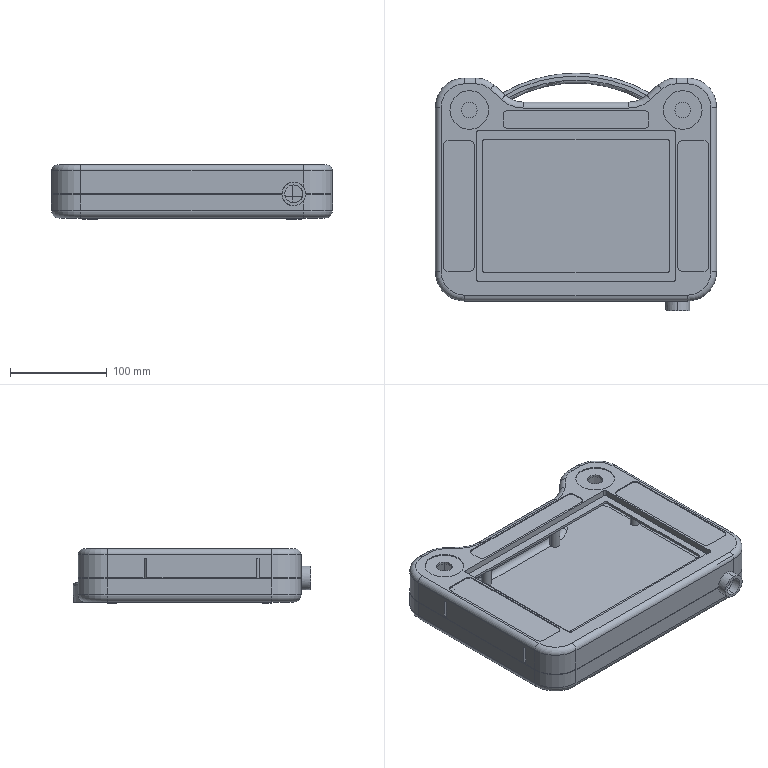Part | STEP file | 1 solid | 1228 faces | box 290 x 245 x 56 mm | volume 381132 mm3 | sphere 756 | cylinder 227 | plane 203 | torus 36 | cone 6 | commonest cylinder face diameters 10 x32 4 x24 2.6 x16 6 x16 15 x15 16 x14